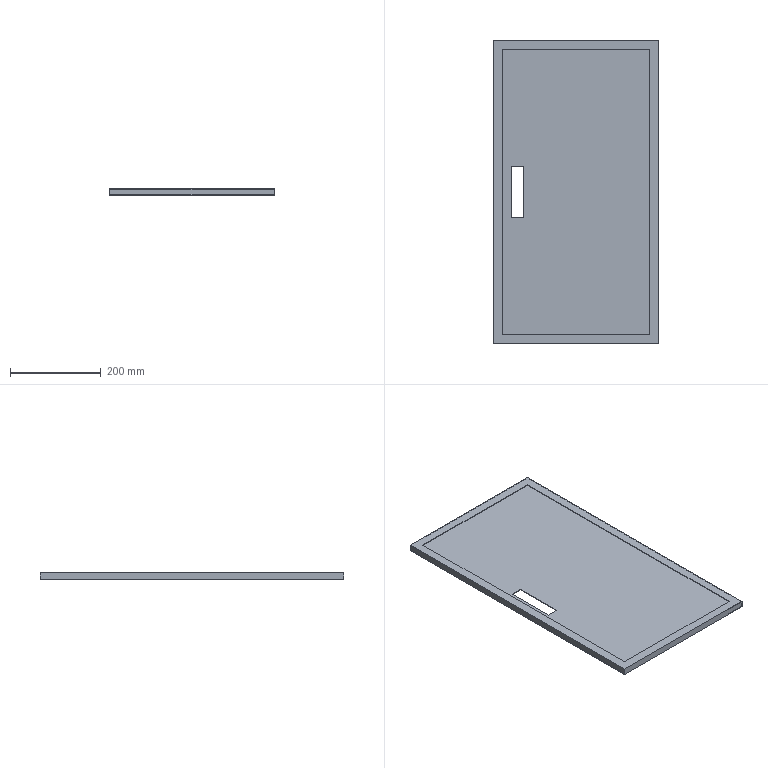Part | SolidWorks | features MirrorStock 1 | 1 solid | 20 faces | box 366 x 670 x 15 mm | volume 460286 mm3 | plane 20
STEP:
#1=CARTESIAN_POINT('',(183.,-335.,0.));
#2=VERTEX_POINT('',#1);
#3=CARTESIAN_POINT('',(183.,335.,0.));
#4=VERTEX_POINT('',#3);
#5=CARTESIAN_POINT('',(183.,-335.,0.));
#6=DIRECTION('',(0.,1.,0.));
#7=VECTOR('',#6,1000.);
#8=LINE('',#5,#7);
#9=EDGE_CURVE('',#2,#4,#8,.T.);
#10=ORIENTED_EDGE('',*,*,#9,.T.);
#11=CARTESIAN_POINT('',(-183.,335.,0.));
#12=VERTEX_POINT('',#11);
#13=CARTESIAN_POINT('',(-183.,335.,0.));
#14=DIRECTION('',(-1.,0.,0.));
#15=VECTOR('',#14,1000.);
#16=LINE('',#13,#15);
#17=EDGE_CURVE('',#4,#12,#16,.T.);
#18=ORIENTED_EDGE('',*,*,#17,.T.);
#19=CARTESIAN_POINT('',(-183.,-335.,0.));
#20=VERTEX_POINT('',#19);
#21=CARTESIAN_POINT('',(-183.,-335.,0.));
#22=DIRECTION('',(0.,-1.,0.));
#23=VECTOR('',#22,1000.);
#24=LINE('',#21,#23);
#25=EDGE_CURVE('',#12,#20,#24,.T.);
#26=ORIENTED_EDGE('',*,*,#25,.T.);
#27=CARTESIAN_POINT('',(-183.,-335.,0.));
#28=DIRECTION('',(1.,0.,0.));
#29=VECTOR('',#28,1000.);
#30=LINE('',#27,#29);
#31=EDGE_CURVE('',#20,#2,#30,.T.);
#32=ORIENTED_EDGE('',*,*,#31,.T.);
#33=EDGE_LOOP('',(#10,#18,#26,#32));
#34=FACE_OUTER_BOUND('',#33,.T.);
#35=CARTESIAN_POINT('',(163.,-315.,0.));
#36=VERTEX_POINT('',#35);
#37=CARTESIAN_POINT('',(-163.,-315.,0.));
#38=VERTEX_POINT('',#37);
#39=CARTESIAN_POINT('',(163.,-315.,0.));
#40=DIRECTION('',(-1.,0.,0.));
#41=VECTOR('',#40,1000.);
#42=LINE('',#39,#41);
#43=EDGE_CURVE('',#36,#38,#42,.T.);
#44=ORIENTED_EDGE('',*,*,#43,.T.);
#45=CARTESIAN_POINT('',(-163.,315.,0.));
#46=VERTEX_POINT('',#45);
#47=CARTESIAN_POINT('',(-163.,-315.,0.));
#48=DIRECTION('',(0.,1.,0.));
#49=VECTOR('',#48,1000.);
#50=LINE('',#47,#49);
#51=EDGE_CURVE('',#38,#46,#50,.T.);
#52=ORIENTED_EDGE('',*,*,#51,.T.);
#53=CARTESIAN_POINT('',(163.,315.,0.));
#54=VERTEX_POINT('',#53);
#55=CARTESIAN_POINT('',(163.,315.,0.));
#56=DIRECTION('',(-1.,0.,0.));
#57=VECTOR('',#56,1000.);
#58=LINE('',#55,#57);
#59=EDGE_CURVE('',#54,#46,#58,.T.);
#60=ORIENTED_EDGE('',*,*,#59,.F.);
#61=CARTESIAN_POINT('',(163.,-315.,0.));
#62=DIRECTION('',(0.,1.,0.));
#63=VECTOR('',#62,1000.);
#64=LINE('',#61,#63);
#65=EDGE_CURVE('',#36,#54,#64,.T.);
#66=ORIENTED_EDGE('',*,*,#65,.F.);
#67=EDGE_LOOP('',(#44,#52,#60,#66));
#68=FACE_BOUND('',#67,.T.);
#69=CARTESIAN_POINT('',(0.,0.,0.));
#70=DIRECTION('',(0.,0.,1.));
#71=DIRECTION('',(-1.,0.,0.));
#72=AXIS2_PLACEMENT_3D('',#69,#70,#71);
#73=PLANE('',#72);
#74=ADVANCED_FACE('',(#34,#68),#73,.T.);
#75=ORIENTED_EDGE('',*,*,#9,.F.);
#76=CARTESIAN_POINT('',(183.,-335.,-15.));
#77=VERTEX_POINT('',#76);
#78=CARTESIAN_POINT('',(183.,-335.,-15.));
#79=DIRECTION('',(0.,0.,1.));
#80=VECTOR('',#79,1000.);
#81=LINE('',#78,#80);
#82=EDGE_CURVE('',#77,#2,#81,.T.);
#83=ORIENTED_EDGE('',*,*,#82,.F.);
#84=CARTESIAN_POINT('',(183.,335.,-15.));
#85=VERTEX_POINT('',#84);
#86=CARTESIAN_POINT('',(183.,-335.,-15.));
#87=DIRECTION('',(0.,1.,0.));
#88=VECTOR('',#87,1000.);
#89=LINE('',#86,#88);
#90=EDGE_CURVE('',#77,#85,#89,.T.);
#91=ORIENTED_EDGE('',*,*,#90,.T.);
#92=CARTESIAN_POINT('',(183.,335.,-15.));
#93=DIRECTION('',(0.,0.,1.));
#94=VECTOR('',#93,1000.);
#95=LINE('',#92,#94);
#96=EDGE_CURVE('',#85,#4,#95,.T.);
#97=ORIENTED_EDGE('',*,*,#96,.T.);
#98=EDGE_LOOP('',(#75,#83,#91,#97));
#99=FACE_OUTER_BOUND('',#98,.T.);
#100=CARTESIAN_POINT('',(183.,-335.,-15.));
#101=DIRECTION('',(-1.,0.,0.));
#102=DIRECTION('',(0.,0.,-1.));
#103=AXIS2_PLACEMENT_3D('',#100,#101,#102);
#104=PLANE('',#103);
#105=ADVANCED_FACE('',(#99),#104,.F.);
#106=ORIENTED_EDGE('',*,*,#17,.F.);
#107=ORIENTED_EDGE('',*,*,#96,.F.);
#108=CARTESIAN_POINT('',(-183.,335.,-15.));
#109=VERTEX_POINT('',#108);
#110=CARTESIAN_POINT('',(-183.,335.,-15.));
#111=DIRECTION('',(-1.,0.,0.));
#112=VECTOR('',#111,1000.);
#113=LINE('',#110,#112);
#114=EDGE_CURVE('',#85,#109,#113,.T.);
#115=ORIENTED_EDGE('',*,*,#114,.T.);
#116=CARTESIAN_POINT('',(-183.,335.,-15.));
#117=DIRECTION('',(0.,0.,1.));
#118=VECTOR('',#117,1000.);
#119=LINE('',#116,#118);
#120=EDGE_CURVE('',#109,#12,#119,.T.);
#121=ORIENTED_EDGE('',*,*,#120,.T.);
#122=EDGE_LOOP('',(#106,#107,#115,#121));
#123=FACE_OUTER_BOUND('',#122,.T.);
#124=CARTESIAN_POINT('',(-183.,335.,-15.));
#125=DIRECTION('',(0.,-1.,0.));
#126=DIRECTION('',(0.,0.,1.));
#127=AXIS2_PLACEMENT_3D('',#124,#125,#126);
#128=PLANE('',#127);
#129=ADVANCED_FACE('',(#123),#128,.F.);
#130=ORIENTED_EDGE('',*,*,#25,.F.);
#131=ORIENTED_EDGE('',*,*,#120,.F.);
#132=CARTESIAN_POINT('',(-183.,-335.,-15.));
#133=VERTEX_POINT('',#132);
#134=CARTESIAN_POINT('',(-183.,-335.,-15.));
#135=DIRECTION('',(0.,-1.,0.));
#136=VECTOR('',#135,1000.);
#137=LINE('',#134,#136);
#138=EDGE_CURVE('',#109,#133,#137,.T.);
#139=ORIENTED_EDGE('',*,*,#138,.T.);
#140=CARTESIAN_POINT('',(-183.,-335.,-15.));
#141=DIRECTION('',(0.,0.,1.));
#142=VECTOR('',#141,1000.);
#143=LINE('',#140,#142);
#144=EDGE_CURVE('',#133,#20,#143,.T.);
#145=ORIENTED_EDGE('',*,*,#144,.T.);
#146=EDGE_LOOP('',(#130,#131,#139,#145));
#147=FACE_OUTER_BOUND('',#146,.T.);
#148=CARTESIAN_POINT('',(-183.,-335.,-15.));
#149=DIRECTION('',(1.,0.,0.));
#150=DIRECTION('',(0.,0.,1.));
#151=AXIS2_PLACEMENT_3D('',#148,#149,#150);
#152=PLANE('',#151);
#153=ADVANCED_FACE('',(#147),#152,.F.);
#154=ORIENTED_EDGE('',*,*,#31,.F.);
#155=ORIENTED_EDGE('',*,*,#144,.F.);
#156=CARTESIAN_POINT('',(-183.,-335.,-15.));
#157=DIRECTION('',(1.,0.,0.));
#158=VECTOR('',#157,1000.);
#159=LINE('',#156,#158);
#160=EDGE_CURVE('',#133,#77,#159,.T.);
#161=ORIENTED_EDGE('',*,*,#160,.T.);
#162=ORIENTED_EDGE('',*,*,#82,.T.);
#163=EDGE_LOOP('',(#154,#155,#161,#162));
#164=FACE_OUTER_BOUND('',#163,.T.);
#165=CARTESIAN_POINT('',(-183.,-335.,-15.));
#166=DIRECTION('',(0.,1.,0.));
#167=DIRECTION('',(0.,0.,-1.));
#168=AXIS2_PLACEMENT_3D('',#165,#166,#167);
#169=PLANE('',#168);
#170=ADVANCED_FACE('',(#164),#169,.F.);
#171=CARTESIAN_POINT('',(-142.75,-56.5,-15.));
#172=VERTEX_POINT('',#171);
#173=CARTESIAN_POINT('',(-116.25,-56.5,-15.));
#174=VERTEX_POINT('',#173);
#175=CARTESIAN_POINT('',(-116.25,-56.5,-15.));
#176=DIRECTION('',(1.,0.,0.));
#177=VECTOR('',#176,1000.);
#178=LINE('',#175,#177);
#179=EDGE_CURVE('',#172,#174,#178,.T.);
#180=ORIENTED_EDGE('',*,*,#179,.T.);
#181=CARTESIAN_POINT('',(-116.25,56.5,-15.));
#182=VERTEX_POINT('',#181);
#183=CARTESIAN_POINT('',(-116.25,-56.5,-15.));
#184=DIRECTION('',(0.,1.,0.));
#185=VECTOR('',#184,1000.);
#186=LINE('',#183,#185);
#187=EDGE_CURVE('',#174,#182,#186,.T.);
#188=ORIENTED_EDGE('',*,*,#187,.T.);
#189=CARTESIAN_POINT('',(-142.75,56.5,-15.));
#190=VERTEX_POINT('',#189);
#191=CARTESIAN_POINT('',(-116.25,56.5,-15.));
#192=DIRECTION('',(-1.,0.,0.));
#193=VECTOR('',#192,1000.);
#194=LINE('',#191,#193);
#195=EDGE_CURVE('',#182,#190,#194,.T.);
#196=ORIENTED_EDGE('',*,*,#195,.T.);
#197=CARTESIAN_POINT('',(-142.75,-56.5,-15.));
#198=DIRECTION('',(0.,-1.,0.));
#199=VECTOR('',#198,1000.);
#200=LINE('',#197,#199);
#201=EDGE_CURVE('',#190,#172,#200,.T.);
#202=ORIENTED_EDGE('',*,*,#201,.T.);
#203=EDGE_LOOP('',(#180,#188,#196,#202));
#204=FACE_BOUND('',#203,.T.);
#205=ORIENTED_EDGE('',*,*,#90,.F.);
#206=ORIENTED_EDGE('',*,*,#160,.F.);
#207=ORIENTED_EDGE('',*,*,#138,.F.);
#208=ORIENTED_EDGE('',*,*,#114,.F.);
#209=EDGE_LOOP('',(#205,#206,#207,#208));
#210=FACE_OUTER_BOUND('',#209,.T.);
#211=CARTESIAN_POINT('',(0.,0.,-15.));
#212=DIRECTION('',(0.,0.,1.));
#213=DIRECTION('',(-1.,0.,0.));
#214=AXIS2_PLACEMENT_3D('',#211,#212,#213);
#215=PLANE('',#214);
#216=ADVANCED_FACE('',(#204,#210),#215,.F.);
#217=ORIENTED_EDGE('',*,*,#65,.T.);
#218=CARTESIAN_POINT('',(163.,315.,-1.5));
#219=VERTEX_POINT('',#218);
#220=CARTESIAN_POINT('',(163.,315.,-1.5));
#221=DIRECTION('',(0.,0.,1.));
#222=VECTOR('',#221,1000.);
#223=LINE('',#220,#222);
#224=EDGE_CURVE('',#219,#54,#223,.T.);
#225=ORIENTED_EDGE('',*,*,#224,.F.);
#226=CARTESIAN_POINT('',(163.,-315.,-1.5));
#227=VERTEX_POINT('',#226);
#228=CARTESIAN_POINT('',(163.,-315.,-1.5));
#229=DIRECTION('',(0.,1.,0.));
#230=VECTOR('',#229,1000.);
#231=LINE('',#228,#230);
#232=EDGE_CURVE('',#227,#219,#231,.T.);
#233=ORIENTED_EDGE('',*,*,#232,.F.);
#234=CARTESIAN_POINT('',(163.,-315.,-1.5));
#235=DIRECTION('',(0.,0.,1.));
#236=VECTOR('',#235,1000.);
#237=LINE('',#234,#236);
#238=EDGE_CURVE('',#227,#36,#237,.T.);
#239=ORIENTED_EDGE('',*,*,#238,.T.);
#240=EDGE_LOOP('',(#217,#225,#233,#239));
#241=FACE_OUTER_BOUND('',#240,.T.);
#242=CARTESIAN_POINT('',(163.,-315.,-1.5));
#243=DIRECTION('',(-1.,0.,0.));
#244=DIRECTION('',(0.,0.,-1.));
#245=AXIS2_PLACEMENT_3D('',#242,#243,#244);
#246=PLANE('',#245);
#247=ADVANCED_FACE('',(#241),#246,.T.);
#248=ORIENTED_EDGE('',*,*,#59,.T.);
#249=CARTESIAN_POINT('',(-163.,315.,-1.5));
#250=VERTEX_POINT('',#249);
#251=CARTESIAN_POINT('',(-163.,315.,-1.5));
#252=DIRECTION('',(0.,0.,1.));
#253=VECTOR('',#252,1000.);
#254=LINE('',#251,#253);
#255=EDGE_CURVE('',#250,#46,#254,.T.);
#256=ORIENTED_EDGE('',*,*,#255,.F.);
#257=CARTESIAN_POINT('',(163.,315.,-1.5));
#258=DIRECTION('',(-1.,0.,0.));
#259=VECTOR('',#258,1000.);
#260=LINE('',#257,#259);
#261=EDGE_CURVE('',#219,#250,#260,.T.);
#262=ORIENTED_EDGE('',*,*,#261,.F.);
#263=ORIENTED_EDGE('',*,*,#224,.T.);
#264=EDGE_LOOP('',(#248,#256,#262,#263));
#265=FACE_OUTER_BOUND('',#264,.T.);
#266=CARTESIAN_POINT('',(163.,315.,-1.5));
#267=DIRECTION('',(0.,-1.,0.));
#268=DIRECTION('',(0.,0.,1.));
#269=AXIS2_PLACEMENT_3D('',#266,#267,#268);
#270=PLANE('',#269);
#271=ADVANCED_FACE('',(#265),#270,.T.);
#272=ORIENTED_EDGE('',*,*,#51,.F.);
#273=CARTESIAN_POINT('',(-163.,-315.,-1.5));
#274=VERTEX_POINT('',#273);
#275=CARTESIAN_POINT('',(-163.,-315.,-1.5));
#276=DIRECTION('',(0.,0.,1.));
#277=VECTOR('',#276,1000.);
#278=LINE('',#275,#277);
#279=EDGE_CURVE('',#274,#38,#278,.T.);
#280=ORIENTED_EDGE('',*,*,#279,.F.);
#281=CARTESIAN_POINT('',(-163.,-315.,-1.5));
#282=DIRECTION('',(0.,1.,0.));
#283=VECTOR('',#282,1000.);
#284=LINE('',#281,#283);
#285=EDGE_CURVE('',#274,#250,#284,.T.);
#286=ORIENTED_EDGE('',*,*,#285,.T.);
#287=ORIENTED_EDGE('',*,*,#255,.T.);
#288=EDGE_LOOP('',(#272,#280,#286,#287));
#289=FACE_OUTER_BOUND('',#288,.T.);
#290=CARTESIAN_POINT('',(-163.,-315.,-1.5));
#291=DIRECTION('',(-1.,0.,0.));
#292=DIRECTION('',(0.,0.,-1.));
#293=AXIS2_PLACEMENT_3D('',#290,#291,#292);
#294=PLANE('',#293);
#295=ADVANCED_FACE('',(#289),#294,.F.);
#296=ORIENTED_EDGE('',*,*,#43,.F.);
#297=ORIENTED_EDGE('',*,*,#238,.F.);
#298=CARTESIAN_POINT('',(163.,-315.,-1.5));
#299=DIRECTION('',(-1.,0.,0.));
#300=VECTOR('',#299,1000.);
#301=LINE('',#298,#300);
#302=EDGE_CURVE('',#227,#274,#301,.T.);
#303=ORIENTED_EDGE('',*,*,#302,.T.);
#304=ORIENTED_EDGE('',*,*,#279,.T.);
#305=EDGE_LOOP('',(#296,#297,#303,#304));
#306=FACE_OUTER_BOUND('',#305,.T.);
#307=CARTESIAN_POINT('',(163.,-315.,-1.5));
#308=DIRECTION('',(0.,-1.,0.));
#309=DIRECTION('',(0.,0.,1.));
#310=AXIS2_PLACEMENT_3D('',#307,#308,#309);
#311=PLANE('',#310);
#312=ADVANCED_FACE('',(#306),#311,.F.);
#313=CARTESIAN_POINT('',(181.5,-333.5,-1.5));
#314=VERTEX_POINT('',#313);
#315=CARTESIAN_POINT('',(181.5,333.5,-1.5));
#316=VERTEX_POINT('',#315);
#317=CARTESIAN_POINT('',(181.5,0.,-1.5));
#318=DIRECTION('',(0.,1.,0.));
#319=VECTOR('',#318,1000.);
#320=LINE('',#317,#319);
#321=EDGE_CURVE('',#314,#316,#320,.T.);
#322=ORIENTED_EDGE('',*,*,#321,.F.);
#323=CARTESIAN_POINT('',(-181.5,-333.5,-1.5));
#324=VERTEX_POINT('',#323);
#325=CARTESIAN_POINT('',(0.,-333.5,-1.5));
#326=DIRECTION('',(1.,0.,0.));
#327=VECTOR('',#326,1000.);
#328=LINE('',#325,#327);
#329=EDGE_CURVE('',#324,#314,#328,.T.);
#330=ORIENTED_EDGE('',*,*,#329,.F.);
#331=CARTESIAN_POINT('',(-181.5,333.5,-1.5));
#332=VERTEX_POINT('',#331);
#333=CARTESIAN_POINT('',(-181.5,0.,-1.5));
#334=DIRECTION('',(0.,-1.,0.));
#335=VECTOR('',#334,1000.);
#336=LINE('',#333,#335);
#337=EDGE_CURVE('',#332,#324,#336,.T.);
#338=ORIENTED_EDGE('',*,*,#337,.F.);
#339=CARTESIAN_POINT('',(0.,333.5,-1.5));
#340=DIRECTION('',(-1.,0.,0.));
#341=VECTOR('',#340,1000.);
#342=LINE('',#339,#341);
#343=EDGE_CURVE('',#316,#332,#342,.T.);
#344=ORIENTED_EDGE('',*,*,#343,.F.);
#345=EDGE_LOOP('',(#322,#330,#338,#344));
#346=FACE_OUTER_BOUND('',#345,.T.);
#347=ORIENTED_EDGE('',*,*,#302,.F.);
#348=ORIENTED_EDGE('',*,*,#232,.T.);
#349=ORIENTED_EDGE('',*,*,#261,.T.);
#350=ORIENTED_EDGE('',*,*,#285,.F.);
#351=EDGE_LOOP('',(#347,#348,#349,#350));
#352=FACE_BOUND('',#351,.T.);
#353=CARTESIAN_POINT('',(0.,0.,-1.5));
#354=DIRECTION('',(0.,0.,1.));
#355=DIRECTION('',(-1.,0.,0.));
#356=AXIS2_PLACEMENT_3D('',#353,#354,#355);
#357=PLANE('',#356);
#358=ADVANCED_FACE('',(#346,#352),#357,.F.);
#359=ORIENTED_EDGE('',*,*,#321,.T.);
#360=CARTESIAN_POINT('',(181.5,333.5,-13.5));
#361=VERTEX_POINT('',#360);
#362=CARTESIAN_POINT('',(181.5,333.5,-15.));
#363=DIRECTION('',(0.,0.,1.));
#364=VECTOR('',#363,1000.);
#365=LINE('',#362,#364);
#366=EDGE_CURVE('',#361,#316,#365,.T.);
#367=ORIENTED_EDGE('',*,*,#366,.F.);
#368=CARTESIAN_POINT('',(181.5,-333.5,-13.5));
#369=VERTEX_POINT('',#368);
#370=CARTESIAN_POINT('',(181.5,0.,-13.5));
#371=DIRECTION('',(0.,1.,0.));
#372=VECTOR('',#371,1000.);
#373=LINE('',#370,#372);
#374=EDGE_CURVE('',#369,#361,#373,.T.);
#375=ORIENTED_EDGE('',*,*,#374,.F.);
#376=CARTESIAN_POINT('',(181.5,-333.5,-15.));
#377=DIRECTION('',(0.,0.,1.));
#378=VECTOR('',#377,1000.);
#379=LINE('',#376,#378);
#380=EDGE_CURVE('',#369,#314,#379,.T.);
#381=ORIENTED_EDGE('',*,*,#380,.T.);
#382=EDGE_LOOP('',(#359,#367,#375,#381));
#383=FACE_OUTER_BOUND('',#382,.T.);
#384=CARTESIAN_POINT('',(181.5,-335.,-15.));
#385=DIRECTION('',(-1.,0.,0.));
#386=DIRECTION('',(0.,0.,-1.));
#387=AXIS2_PLACEMENT_3D('',#384,#385,#386);
#388=PLANE('',#387);
#389=ADVANCED_FACE('',(#383),#388,.T.);
#390=ORIENTED_EDGE('',*,*,#343,.T.);
#391=CARTESIAN_POINT('',(-181.5,333.5,-13.5));
#392=VERTEX_POINT('',#391);
#393=CARTESIAN_POINT('',(-181.5,333.5,-15.));
#394=DIRECTION('',(0.,0.,1.));
#395=VECTOR('',#394,1000.);
#396=LINE('',#393,#395);
#397=EDGE_CURVE('',#392,#332,#396,.T.);
#398=ORIENTED_EDGE('',*,*,#397,.F.);
#399=CARTESIAN_POINT('',(0.,333.5,-13.5));
#400=DIRECTION('',(-1.,0.,0.));
#401=VECTOR('',#400,1000.);
#402=LINE('',#399,#401);
#403=EDGE_CURVE('',#361,#392,#402,.T.);
#404=ORIENTED_EDGE('',*,*,#403,.F.);
#405=ORIENTED_EDGE('',*,*,#366,.T.);
#406=EDGE_LOOP('',(#390,#398,#404,#405));
#407=FACE_OUTER_BOUND('',#406,.T.);
#408=CARTESIAN_POINT('',(-183.,333.5,-15.));
#409=DIRECTION('',(0.,-1.,0.));
#410=DIRECTION('',(0.,0.,1.));
#411=AXIS2_PLACEMENT_3D('',#408,#409,#410);
#412=PLANE('',#411);
#413=ADVANCED_FACE('',(#407),#412,.T.);
#414=ORIENTED_EDGE('',*,*,#337,.T.);
#415=CARTESIAN_POINT('',(-181.5,-333.5,-13.5));
#416=VERTEX_POINT('',#415);
#417=CARTESIAN_POINT('',(-181.5,-333.5,-15.));
#418=DIRECTION('',(0.,0.,1.));
#419=VECTOR('',#418,1000.);
#420=LINE('',#417,#419);
#421=EDGE_CURVE('',#416,#324,#420,.T.);
#422=ORIENTED_EDGE('',*,*,#421,.F.);
#423=CARTESIAN_POINT('',(-181.5,0.,-13.5));
#424=DIRECTION('',(0.,-1.,0.));
#425=VECTOR('',#424,1000.);
#426=LINE('',#423,#425);
#427=EDGE_CURVE('',#392,#416,#426,.T.);
#428=ORIENTED_EDGE('',*,*,#427,.F.);
#429=ORIENTED_EDGE('',*,*,#397,.T.);
#430=EDGE_LOOP('',(#414,#422,#428,#429));
#431=FACE_OUTER_BOUND('',#430,.T.);
#432=CARTESIAN_POINT('',(-181.5,-335.,-15.));
#433=DIRECTION('',(1.,0.,0.));
#434=DIRECTION('',(0.,0.,1.));
#435=AXIS2_PLACEMENT_3D('',#432,#433,#434);
#436=PLANE('',#435);
#437=ADVANCED_FACE('',(#431),#436,.T.);
#438=ORIENTED_EDGE('',*,*,#329,.T.);
#439=ORIENTED_EDGE('',*,*,#380,.F.);
#440=CARTESIAN_POINT('',(0.,-333.5,-13.5));
#441=DIRECTION('',(1.,0.,0.));
#442=VECTOR('',#441,1000.);
#443=LINE('',#440,#442);
#444=EDGE_CURVE('',#416,#369,#443,.T.);
#445=ORIENTED_EDGE('',*,*,#444,.F.);
#446=ORIENTED_EDGE('',*,*,#421,.T.);
#447=EDGE_LOOP('',(#438,#439,#445,#446));
#448=FACE_OUTER_BOUND('',#447,.T.);
#449=CARTESIAN_POINT('',(-183.,-333.5,-15.));
#450=DIRECTION('',(0.,1.,0.));
#451=DIRECTION('',(0.,0.,-1.));
#452=AXIS2_PLACEMENT_3D('',#449,#450,#451);
#453=PLANE('',#452);
#454=ADVANCED_FACE('',(#448),#453,.T.);
#455=CARTESIAN_POINT('',(-142.75,-56.5,-13.5));
#456=VERTEX_POINT('',#455);
#457=CARTESIAN_POINT('',(-142.75,56.5,-13.5));
#458=VERTEX_POINT('',#457);
#459=CARTESIAN_POINT('',(-142.75,0.,-13.5));
#460=DIRECTION('',(0.,1.,0.));
#461=VECTOR('',#460,1000.);
#462=LINE('',#459,#461);
#463=EDGE_CURVE('',#456,#458,#462,.T.);
#464=ORIENTED_EDGE('',*,*,#463,.T.);
#465=CARTESIAN_POINT('',(-116.25,56.5,-13.5));
#466=VERTEX_POINT('',#465);
#467=CARTESIAN_POINT('',(0.,56.5,-13.5));
#468=DIRECTION('',(1.,0.,0.));
#469=VECTOR('',#468,1000.);
#470=LINE('',#467,#469);
#471=EDGE_CURVE('',#458,#466,#470,.T.);
#472=ORIENTED_EDGE('',*,*,#471,.T.);
#473=CARTESIAN_POINT('',(-116.25,-56.5,-13.5));
#474=VERTEX_POINT('',#473);
#475=CARTESIAN_POINT('',(-116.25,0.,-13.5));
#476=DIRECTION('',(0.,-1.,0.));
#477=VECTOR('',#476,1000.);
#478=LINE('',#475,#477);
#479=EDGE_CURVE('',#466,#474,#478,.T.);
#480=ORIENTED_EDGE('',*,*,#479,.T.);
#481=CARTESIAN_POINT('',(0.,-56.5,-13.5));
#482=DIRECTION('',(-1.,0.,0.));
#483=VECTOR('',#482,1000.);
#484=LINE('',#481,#483);
#485=EDGE_CURVE('',#474,#456,#484,.T.);
#486=ORIENTED_EDGE('',*,*,#485,.T.);
#487=EDGE_LOOP('',(#464,#472,#480,#486));
#488=FACE_BOUND('',#487,.T.);
#489=ORIENTED_EDGE('',*,*,#374,.T.);
#490=ORIENTED_EDGE('',*,*,#403,.T.);
#491=ORIENTED_EDGE('',*,*,#427,.T.);
#492=ORIENTED_EDGE('',*,*,#444,.T.);
#493=EDGE_LOOP('',(#489,#490,#491,#492));
#494=FACE_OUTER_BOUND('',#493,.T.);
#495=CARTESIAN_POINT('',(0.,0.,-13.5));
#496=DIRECTION('',(0.,0.,1.));
#497=DIRECTION('',(-1.,0.,0.));
#498=AXIS2_PLACEMENT_3D('',#495,#496,#497);
#499=PLANE('',#498);
#500=ADVANCED_FACE('',(#488,#494),#499,.T.);
#501=ORIENTED_EDGE('',*,*,#463,.F.);
#502=CARTESIAN_POINT('',(-142.75,-56.5,-12.));
#503=DIRECTION('',(0.,0.,-1.));
#504=VECTOR('',#503,1000.);
#505=LINE('',#502,#504);
#506=EDGE_CURVE('',#456,#172,#505,.T.);
#507=ORIENTED_EDGE('',*,*,#506,.T.);
#508=ORIENTED_EDGE('',*,*,#201,.F.);
#509=CARTESIAN_POINT('',(-142.75,56.5,-12.));
#510=DIRECTION('',(0.,0.,-1.));
#511=VECTOR('',#510,1000.);
#512=LINE('',#509,#511);
#513=EDGE_CURVE('',#458,#190,#512,.T.);
#514=ORIENTED_EDGE('',*,*,#513,.F.);
#515=EDGE_LOOP('',(#501,#507,#508,#514));
#516=FACE_OUTER_BOUND('',#515,.T.);
#517=CARTESIAN_POINT('',(-142.75,-56.5,-12.));
#518=DIRECTION('',(-1.,0.,0.));
#519=DIRECTION('',(0.,0.,-1.));
#520=AXIS2_PLACEMENT_3D('',#517,#518,#519);
#521=PLANE('',#520);
#522=ADVANCED_FACE('',(#516),#521,.F.);
#523=ORIENTED_EDGE('',*,*,#471,.F.);
#524=ORIENTED_EDGE('',*,*,#513,.T.);
#525=ORIENTED_EDGE('',*,*,#195,.F.);
#526=CARTESIAN_POINT('',(-116.25,56.5,-12.));
#527=DIRECTION('',(0.,0.,-1.));
#528=VECTOR('',#527,1000.);
#529=LINE('',#526,#528);
#530=EDGE_CURVE('',#466,#182,#529,.T.);
#531=ORIENTED_EDGE('',*,*,#530,.F.);
#532=EDGE_LOOP('',(#523,#524,#525,#531));
#533=FACE_OUTER_BOUND('',#532,.T.);
#534=CARTESIAN_POINT('',(-116.25,56.5,-12.));
#535=DIRECTION('',(0.,1.,0.));
#536=DIRECTION('',(-1.,0.,0.));
#537=AXIS2_PLACEMENT_3D('',#534,#535,#536);
#538=PLANE('',#537);
#539=ADVANCED_FACE('',(#533),#538,.F.);
#540=ORIENTED_EDGE('',*,*,#479,.F.);
#541=ORIENTED_EDGE('',*,*,#530,.T.);
#542=ORIENTED_EDGE('',*,*,#187,.F.);
#543=CARTESIAN_POINT('',(-116.25,-56.5,-12.));
#544=DIRECTION('',(0.,0.,-1.));
#545=VECTOR('',#544,1000.);
#546=LINE('',#543,#545);
#547=EDGE_CURVE('',#474,#174,#546,.T.);
#548=ORIENTED_EDGE('',*,*,#547,.F.);
#549=EDGE_LOOP('',(#540,#541,#542,#548));
#550=FACE_OUTER_BOUND('',#549,.T.);
#551=CARTESIAN_POINT('',(-116.25,-56.5,-12.));
#552=DIRECTION('',(1.,0.,0.));
#553=DIRECTION('',(0.,0.,1.));
#554=AXIS2_PLACEMENT_3D('',#551,#552,#553);
#555=PLANE('',#554);
#556=ADVANCED_FACE('',(#550),#555,.F.);
#557=ORIENTED_EDGE('',*,*,#485,.F.);
#558=ORIENTED_EDGE('',*,*,#547,.T.);
#559=ORIENTED_EDGE('',*,*,#179,.F.);
#560=ORIENTED_EDGE('',*,*,#506,.F.);
#561=EDGE_LOOP('',(#557,#558,#559,#560));
#562=FACE_OUTER_BOUND('',#561,.T.);
#563=CARTESIAN_POINT('',(-116.25,-56.5,-12.));
#564=DIRECTION('',(0.,-1.,0.));
#565=DIRECTION('',(1.,0.,0.));
#566=AXIS2_PLACEMENT_3D('',#563,#564,#565);
#567=PLANE('',#566);
#568=ADVANCED_FACE('',(#562),#567,.F.);
#569=CLOSED_SHELL('',(#74,#105,#129,#153,#170,#216,#247,#271,#295,#312,#358,#389,#413,#437,#454,#500,#522,#539,#556,#568));
#570=MANIFOLD_SOLID_BREP('',#569);
#571=CARTESIAN_POINT('',(0.,0.,0.));
#572=DIRECTION('',(0.,0.,1.));
#573=DIRECTION('',(1.,0.,0.));
#574=AXIS2_PLACEMENT_3D('',#571,#572,#573);
#575=(LENGTH_UNIT()NAMED_UNIT(*)SI_UNIT(.MILLI.,.METRE.));
#576=UNCERTAINTY_MEASURE_WITH_UNIT(LENGTH_MEASURE(0.00001),#575,'','');
#577=(NAMED_UNIT(*)PLANE_ANGLE_UNIT()SI_UNIT($,.RADIAN.));
#578=(NAMED_UNIT(*)SI_UNIT($,.STERADIAN.)SOLID_ANGLE_UNIT());
#579=(GEOMETRIC_REPRESENTATION_CONTEXT(3)GLOBAL_UNCERTAINTY_ASSIGNED_CONTEXT((#576))GLOBAL_UNIT_ASSIGNED_CONTEXT((#575,#577,#578))REPRESENTATION_CONTEXT('',''));
#580=ADVANCED_BREP_SHAPE_REPRESENTATION('',(#570,#574),#579);